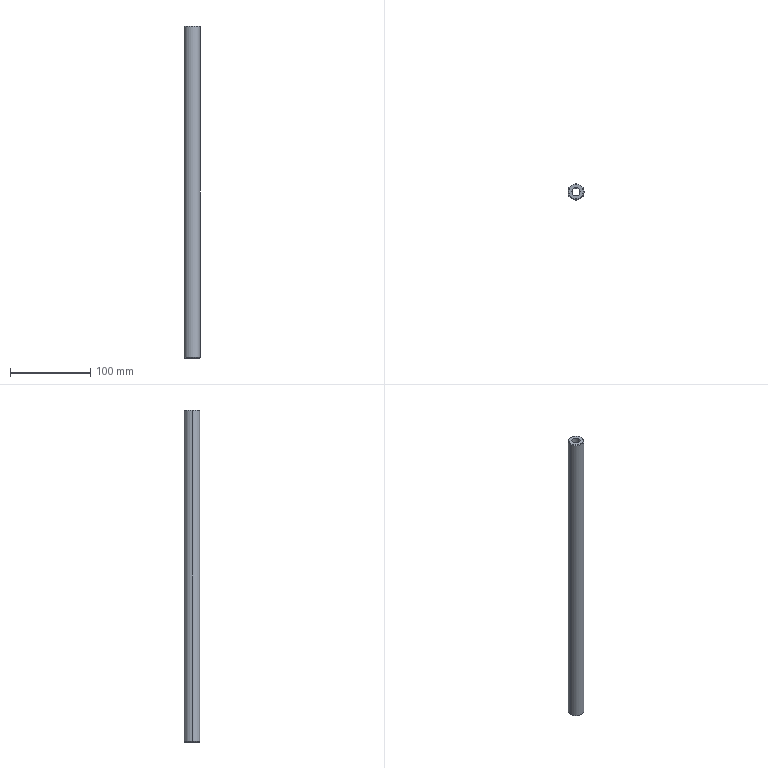Part | SolidWorks | features HoleWzd 2, Revolution 1 | 1 solid | 10 faces | box 20 x 20 x 415 mm | volume 96405 mm3 | cylinder 4 | cone 4 | plane 2 | commonest cylinder face diameters 10.2 x2 20 x2
STEP:
#1=CARTESIAN_POINT('',(-5.1,0.,207.5));
#2=VERTEX_POINT('',#1);
#3=CARTESIAN_POINT('',(5.1,0.,207.5));
#4=VERTEX_POINT('',#3);
#5=CARTESIAN_POINT('',(0.,0.,207.5));
#6=DIRECTION('',(0.,0.,1.));
#7=DIRECTION('',(1.,0.,0.));
#8=AXIS2_PLACEMENT_3D('',#5,#6,#7);
#9=CIRCLE('',#8,5.1);
#10=EDGE_CURVE('',#2,#4,#9,.T.);
#11=ORIENTED_EDGE('',*,*,#10,.T.);
#12=CARTESIAN_POINT('',(5.1,0.,-207.5));
#13=VERTEX_POINT('',#12);
#14=CARTESIAN_POINT('',(5.1,0.,-207.5));
#15=DIRECTION('',(0.,0.,-1.));
#16=VECTOR('',#15,1000.);
#17=LINE('',#14,#16);
#18=EDGE_CURVE('',#4,#13,#17,.T.);
#19=ORIENTED_EDGE('',*,*,#18,.T.);
#20=CARTESIAN_POINT('',(-5.1,0.,-207.5));
#21=VERTEX_POINT('',#20);
#22=CARTESIAN_POINT('',(0.,0.,-207.5));
#23=DIRECTION('',(0.,0.,-1.));
#24=DIRECTION('',(-1.,0.,0.));
#25=AXIS2_PLACEMENT_3D('',#22,#23,#24);
#26=CIRCLE('',#25,5.1);
#27=EDGE_CURVE('',#13,#21,#26,.T.);
#28=ORIENTED_EDGE('',*,*,#27,.T.);
#29=CARTESIAN_POINT('',(-5.1,0.,-207.5));
#30=DIRECTION('',(0.,0.,-1.));
#31=VECTOR('',#30,1000.);
#32=LINE('',#29,#31);
#33=EDGE_CURVE('',#2,#21,#32,.T.);
#34=ORIENTED_EDGE('',*,*,#33,.F.);
#35=EDGE_LOOP('',(#11,#19,#28,#34));
#36=FACE_OUTER_BOUND('',#35,.T.);
#37=CARTESIAN_POINT('',(0.,0.,-207.5));
#38=DIRECTION('',(0.,0.,-1.));
#39=DIRECTION('',(-1.,0.,0.));
#40=AXIS2_PLACEMENT_3D('',#37,#38,#39);
#41=CYLINDRICAL_SURFACE('',#40,5.1);
#42=ADVANCED_FACE('',(#36),#41,.F.);
#43=CARTESIAN_POINT('',(-9.,0.,207.5));
#44=VERTEX_POINT('',#43);
#45=CARTESIAN_POINT('',(9.,0.,207.5));
#46=VERTEX_POINT('',#45);
#47=CARTESIAN_POINT('',(0.,0.,207.5));
#48=DIRECTION('',(0.,0.,-1.));
#49=DIRECTION('',(-1.,0.,0.));
#50=AXIS2_PLACEMENT_3D('',#47,#48,#49);
#51=CIRCLE('',#50,9.);
#52=EDGE_CURVE('',#44,#46,#51,.T.);
#53=ORIENTED_EDGE('',*,*,#52,.T.);
#54=CARTESIAN_POINT('',(10.,0.,206.5));
#55=VERTEX_POINT('',#54);
#56=CARTESIAN_POINT('',(10.,0.,206.5));
#57=DIRECTION('',(0.7071,0.,-0.7071));
#58=VECTOR('',#57,1000.);
#59=LINE('',#56,#58);
#60=EDGE_CURVE('',#46,#55,#59,.T.);
#61=ORIENTED_EDGE('',*,*,#60,.T.);
#62=CARTESIAN_POINT('',(-10.,0.,206.5));
#63=VERTEX_POINT('',#62);
#64=CARTESIAN_POINT('',(0.,0.,206.5));
#65=DIRECTION('',(0.,0.,-1.));
#66=DIRECTION('',(-1.,0.,0.));
#67=AXIS2_PLACEMENT_3D('',#64,#65,#66);
#68=CIRCLE('',#67,10.);
#69=EDGE_CURVE('',#63,#55,#68,.T.);
#70=ORIENTED_EDGE('',*,*,#69,.F.);
#71=CARTESIAN_POINT('',(-10.,0.,206.5));
#72=DIRECTION('',(-0.7071,0.,-0.7071));
#73=VECTOR('',#72,1000.);
#74=LINE('',#71,#73);
#75=EDGE_CURVE('',#44,#63,#74,.T.);
#76=ORIENTED_EDGE('',*,*,#75,.F.);
#77=EDGE_LOOP('',(#53,#61,#70,#76));
#78=FACE_OUTER_BOUND('',#77,.T.);
#79=CARTESIAN_POINT('',(0.,0.,206.5));
#80=DIRECTION('',(0.,0.,-1.));
#81=DIRECTION('',(-1.,0.,0.));
#82=AXIS2_PLACEMENT_3D('',#79,#80,#81);
#83=CONICAL_SURFACE('',#82,10.,0.7854);
#84=ADVANCED_FACE('',(#78),#83,.T.);
#85=ORIENTED_EDGE('',*,*,#69,.T.);
#86=CARTESIAN_POINT('',(10.,0.,-206.5));
#87=VERTEX_POINT('',#86);
#88=CARTESIAN_POINT('',(10.,0.,207.5));
#89=DIRECTION('',(0.,0.,-1.));
#90=VECTOR('',#89,1000.);
#91=LINE('',#88,#90);
#92=EDGE_CURVE('',#55,#87,#91,.T.);
#93=ORIENTED_EDGE('',*,*,#92,.T.);
#94=CARTESIAN_POINT('',(-10.,0.,-206.5));
#95=VERTEX_POINT('',#94);
#96=CARTESIAN_POINT('',(0.,0.,-206.5));
#97=DIRECTION('',(0.,0.,-1.));
#98=DIRECTION('',(-1.,0.,0.));
#99=AXIS2_PLACEMENT_3D('',#96,#97,#98);
#100=CIRCLE('',#99,10.);
#101=EDGE_CURVE('',#95,#87,#100,.T.);
#102=ORIENTED_EDGE('',*,*,#101,.F.);
#103=CARTESIAN_POINT('',(-10.,0.,207.5));
#104=DIRECTION('',(0.,0.,-1.));
#105=VECTOR('',#104,1000.);
#106=LINE('',#103,#105);
#107=EDGE_CURVE('',#63,#95,#106,.T.);
#108=ORIENTED_EDGE('',*,*,#107,.F.);
#109=EDGE_LOOP('',(#85,#93,#102,#108));
#110=FACE_OUTER_BOUND('',#109,.T.);
#111=CARTESIAN_POINT('',(0.,0.,207.5));
#112=DIRECTION('',(0.,0.,-1.));
#113=DIRECTION('',(-1.,0.,0.));
#114=AXIS2_PLACEMENT_3D('',#111,#112,#113);
#115=CYLINDRICAL_SURFACE('',#114,10.);
#116=ADVANCED_FACE('',(#110),#115,.T.);
#117=CARTESIAN_POINT('',(-9.,0.,-207.5));
#118=VERTEX_POINT('',#117);
#119=CARTESIAN_POINT('',(9.,0.,-207.5));
#120=VERTEX_POINT('',#119);
#121=CARTESIAN_POINT('',(0.,0.,-207.5));
#122=DIRECTION('',(0.,0.,-1.));
#123=DIRECTION('',(-1.,0.,0.));
#124=AXIS2_PLACEMENT_3D('',#121,#122,#123);
#125=CIRCLE('',#124,9.);
#126=EDGE_CURVE('',#118,#120,#125,.T.);
#127=ORIENTED_EDGE('',*,*,#126,.F.);
#128=CARTESIAN_POINT('',(-9.,0.,-207.5));
#129=DIRECTION('',(-0.7071,0.,0.7071));
#130=VECTOR('',#129,1000.);
#131=LINE('',#128,#130);
#132=EDGE_CURVE('',#118,#95,#131,.T.);
#133=ORIENTED_EDGE('',*,*,#132,.T.);
#134=ORIENTED_EDGE('',*,*,#101,.T.);
#135=CARTESIAN_POINT('',(9.,0.,-207.5));
#136=DIRECTION('',(0.7071,0.,0.7071));
#137=VECTOR('',#136,1000.);
#138=LINE('',#135,#137);
#139=EDGE_CURVE('',#120,#87,#138,.T.);
#140=ORIENTED_EDGE('',*,*,#139,.F.);
#141=EDGE_LOOP('',(#127,#133,#134,#140));
#142=FACE_OUTER_BOUND('',#141,.T.);
#143=CARTESIAN_POINT('',(0.,0.,-207.5));
#144=DIRECTION('',(0.,0.,1.));
#145=DIRECTION('',(1.,0.,0.));
#146=AXIS2_PLACEMENT_3D('',#143,#144,#145);
#147=CONICAL_SURFACE('',#146,9.,0.7854);
#148=ADVANCED_FACE('',(#142),#147,.T.);
#149=CARTESIAN_POINT('',(0.,0.,-207.5));
#150=DIRECTION('',(0.,0.,-1.));
#151=DIRECTION('',(-1.,0.,0.));
#152=AXIS2_PLACEMENT_3D('',#149,#150,#151);
#153=CIRCLE('',#152,5.1);
#154=EDGE_CURVE('',#21,#13,#153,.T.);
#155=ORIENTED_EDGE('',*,*,#154,.F.);
#156=ORIENTED_EDGE('',*,*,#27,.F.);
#157=EDGE_LOOP('',(#155,#156));
#158=FACE_BOUND('',#157,.T.);
#159=CARTESIAN_POINT('',(0.,0.,-207.5));
#160=DIRECTION('',(0.,0.,-1.));
#161=DIRECTION('',(-1.,0.,0.));
#162=AXIS2_PLACEMENT_3D('',#159,#160,#161);
#163=CIRCLE('',#162,9.);
#164=EDGE_CURVE('',#120,#118,#163,.T.);
#165=ORIENTED_EDGE('',*,*,#164,.T.);
#166=ORIENTED_EDGE('',*,*,#126,.T.);
#167=EDGE_LOOP('',(#165,#166));
#168=FACE_OUTER_BOUND('',#167,.T.);
#169=CARTESIAN_POINT('',(0.,0.,-207.5));
#170=DIRECTION('',(0.,0.,-1.));
#171=DIRECTION('',(-1.,0.,0.));
#172=AXIS2_PLACEMENT_3D('',#169,#170,#171);
#173=PLANE('',#172);
#174=ADVANCED_FACE('',(#158,#168),#173,.T.);
#175=ORIENTED_EDGE('',*,*,#132,.F.);
#176=ORIENTED_EDGE('',*,*,#164,.F.);
#177=ORIENTED_EDGE('',*,*,#139,.T.);
#178=CARTESIAN_POINT('',(0.,0.,-206.5));
#179=DIRECTION('',(0.,0.,-1.));
#180=DIRECTION('',(-1.,0.,0.));
#181=AXIS2_PLACEMENT_3D('',#178,#179,#180);
#182=CIRCLE('',#181,10.);
#183=EDGE_CURVE('',#87,#95,#182,.T.);
#184=ORIENTED_EDGE('',*,*,#183,.T.);
#185=EDGE_LOOP('',(#175,#176,#177,#184));
#186=FACE_OUTER_BOUND('',#185,.T.);
#187=CARTESIAN_POINT('',(0.,0.,-207.5));
#188=DIRECTION('',(0.,0.,1.));
#189=DIRECTION('',(1.,0.,0.));
#190=AXIS2_PLACEMENT_3D('',#187,#188,#189);
#191=CONICAL_SURFACE('',#190,9.,0.7854);
#192=ADVANCED_FACE('',(#186),#191,.T.);
#193=ORIENTED_EDGE('',*,*,#92,.F.);
#194=CARTESIAN_POINT('',(0.,0.,206.5));
#195=DIRECTION('',(0.,0.,-1.));
#196=DIRECTION('',(-1.,0.,0.));
#197=AXIS2_PLACEMENT_3D('',#194,#195,#196);
#198=CIRCLE('',#197,10.);
#199=EDGE_CURVE('',#55,#63,#198,.T.);
#200=ORIENTED_EDGE('',*,*,#199,.T.);
#201=ORIENTED_EDGE('',*,*,#107,.T.);
#202=ORIENTED_EDGE('',*,*,#183,.F.);
#203=EDGE_LOOP('',(#193,#200,#201,#202));
#204=FACE_OUTER_BOUND('',#203,.T.);
#205=CARTESIAN_POINT('',(0.,0.,207.5));
#206=DIRECTION('',(0.,0.,-1.));
#207=DIRECTION('',(-1.,0.,0.));
#208=AXIS2_PLACEMENT_3D('',#205,#206,#207);
#209=CYLINDRICAL_SURFACE('',#208,10.);
#210=ADVANCED_FACE('',(#204),#209,.T.);
#211=ORIENTED_EDGE('',*,*,#60,.F.);
#212=CARTESIAN_POINT('',(0.,0.,207.5));
#213=DIRECTION('',(0.,0.,-1.));
#214=DIRECTION('',(-1.,0.,0.));
#215=AXIS2_PLACEMENT_3D('',#212,#213,#214);
#216=CIRCLE('',#215,9.);
#217=EDGE_CURVE('',#46,#44,#216,.T.);
#218=ORIENTED_EDGE('',*,*,#217,.T.);
#219=ORIENTED_EDGE('',*,*,#75,.T.);
#220=ORIENTED_EDGE('',*,*,#199,.F.);
#221=EDGE_LOOP('',(#211,#218,#219,#220));
#222=FACE_OUTER_BOUND('',#221,.T.);
#223=CARTESIAN_POINT('',(0.,0.,206.5));
#224=DIRECTION('',(0.,0.,-1.));
#225=DIRECTION('',(-1.,0.,0.));
#226=AXIS2_PLACEMENT_3D('',#223,#224,#225);
#227=CONICAL_SURFACE('',#226,10.,0.7854);
#228=ADVANCED_FACE('',(#222),#227,.T.);
#229=ORIENTED_EDGE('',*,*,#10,.F.);
#230=CARTESIAN_POINT('',(0.,0.,207.5));
#231=DIRECTION('',(0.,0.,1.));
#232=DIRECTION('',(1.,0.,0.));
#233=AXIS2_PLACEMENT_3D('',#230,#231,#232);
#234=CIRCLE('',#233,5.1);
#235=EDGE_CURVE('',#4,#2,#234,.T.);
#236=ORIENTED_EDGE('',*,*,#235,.F.);
#237=EDGE_LOOP('',(#229,#236));
#238=FACE_BOUND('',#237,.T.);
#239=ORIENTED_EDGE('',*,*,#52,.F.);
#240=ORIENTED_EDGE('',*,*,#217,.F.);
#241=EDGE_LOOP('',(#239,#240));
#242=FACE_OUTER_BOUND('',#241,.T.);
#243=CARTESIAN_POINT('',(9.,0.,207.5));
#244=DIRECTION('',(0.,0.,1.));
#245=DIRECTION('',(1.,0.,0.));
#246=AXIS2_PLACEMENT_3D('',#243,#244,#245);
#247=PLANE('',#246);
#248=ADVANCED_FACE('',(#238,#242),#247,.T.);
#249=ORIENTED_EDGE('',*,*,#18,.F.);
#250=ORIENTED_EDGE('',*,*,#235,.T.);
#251=ORIENTED_EDGE('',*,*,#33,.T.);
#252=ORIENTED_EDGE('',*,*,#154,.T.);
#253=EDGE_LOOP('',(#249,#250,#251,#252));
#254=FACE_OUTER_BOUND('',#253,.T.);
#255=CARTESIAN_POINT('',(0.,0.,-207.5));
#256=DIRECTION('',(0.,0.,-1.));
#257=DIRECTION('',(-1.,0.,0.));
#258=AXIS2_PLACEMENT_3D('',#255,#256,#257);
#259=CYLINDRICAL_SURFACE('',#258,5.1);
#260=ADVANCED_FACE('',(#254),#259,.F.);
#261=CLOSED_SHELL('',(#42,#84,#116,#148,#174,#192,#210,#228,#248,#260));
#262=MANIFOLD_SOLID_BREP('',#261);
#263=CARTESIAN_POINT('',(0.,0.,0.));
#264=DIRECTION('',(0.,0.,1.));
#265=DIRECTION('',(1.,0.,0.));
#266=AXIS2_PLACEMENT_3D('',#263,#264,#265);
#267=(LENGTH_UNIT()NAMED_UNIT(*)SI_UNIT(.MILLI.,.METRE.));
#268=UNCERTAINTY_MEASURE_WITH_UNIT(LENGTH_MEASURE(0.00001),#267,'','');
#269=(NAMED_UNIT(*)PLANE_ANGLE_UNIT()SI_UNIT($,.RADIAN.));
#270=(NAMED_UNIT(*)SI_UNIT($,.STERADIAN.)SOLID_ANGLE_UNIT());
#271=(GEOMETRIC_REPRESENTATION_CONTEXT(3)GLOBAL_UNCERTAINTY_ASSIGNED_CONTEXT((#268))GLOBAL_UNIT_ASSIGNED_CONTEXT((#267,#269,#270))REPRESENTATION_CONTEXT('',''));
#272=ADVANCED_BREP_SHAPE_REPRESENTATION('',(#262,#266),#271);